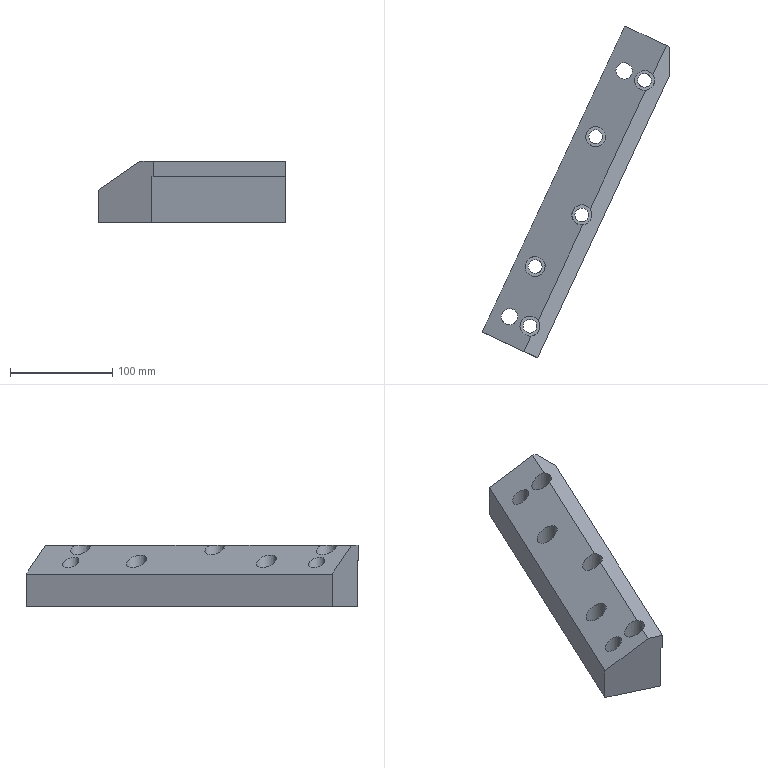Part | NX | features solid 2 | 1 solid | 27 faces | box 183.656 x 324.439 x 60 mm | volume 868161 mm3 | plane 15 | cylinder 12 | commonest cylinder face diameters 13.5 x5 19.5 x5 16 x2
STEP:
#1=CARTESIAN_POINT('',(-201.72,227.591,-65.));
#2=VERTEX_POINT('',#1);
#3=CARTESIAN_POINT('',(-201.72,234.341,-65.));
#4=DIRECTION('',(0.,0.,1.));
#5=DIRECTION('',(0.,-1.,0.));
#6=AXIS2_PLACEMENT_3D('',#3,#4,#5);
#7=CIRCLE('',#6,6.75);
#8=EDGE_CURVE('',#2,#2,#7,.T.);
#9=ORIENTED_EDGE('',*,*,#8,.T.);
#10=EDGE_LOOP('',(#9));
#11=FACE_BOUND('',#10,.T.);
#12=CARTESIAN_POINT('',(-156.124,278.049,-65.));
#13=VERTEX_POINT('',#12);
#14=CARTESIAN_POINT('',(-156.124,284.799,-65.));
#15=DIRECTION('',(0.,0.,1.));
#16=DIRECTION('',(0.,-1.,0.));
#17=AXIS2_PLACEMENT_3D('',#14,#15,#16);
#18=CIRCLE('',#17,6.75);
#19=EDGE_CURVE('',#13,#13,#18,.F.);
#20=ORIENTED_EDGE('',*,*,#19,.F.);
#21=EDGE_LOOP('',(#20));
#22=FACE_BOUND('',#21,.T.);
#23=CARTESIAN_POINT('',(-142.553,354.474,-65.));
#24=VERTEX_POINT('',#23);
#25=CARTESIAN_POINT('',(-142.553,361.224,-65.));
#26=DIRECTION('',(0.,0.,1.));
#27=DIRECTION('',(0.,-1.,0.));
#28=AXIS2_PLACEMENT_3D('',#25,#26,#27);
#29=CIRCLE('',#28,6.75);
#30=EDGE_CURVE('',#24,#24,#29,.F.);
#31=ORIENTED_EDGE('',*,*,#30,.F.);
#32=EDGE_LOOP('',(#31));
#33=FACE_BOUND('',#32,.T.);
#34=CARTESIAN_POINT('',(-94.844,409.463,-65.));
#35=VERTEX_POINT('',#34);
#36=CARTESIAN_POINT('',(-94.844,416.213,-65.));
#37=DIRECTION('',(0.,0.,1.));
#38=DIRECTION('',(0.,-1.,0.));
#39=AXIS2_PLACEMENT_3D('',#36,#37,#38);
#40=CIRCLE('',#39,6.75);
#41=EDGE_CURVE('',#35,#35,#40,.F.);
#42=ORIENTED_EDGE('',*,*,#41,.F.);
#43=EDGE_LOOP('',(#42));
#44=FACE_BOUND('',#43,.T.);
#45=CARTESIAN_POINT('',(-114.783,417.511,-65.));
#46=VERTEX_POINT('',#45);
#47=CARTESIAN_POINT('',(-114.783,425.511,-65.));
#48=DIRECTION('',(0.,0.,1.));
#49=DIRECTION('',(0.,-1.,0.));
#50=AXIS2_PLACEMENT_3D('',#47,#48,#49);
#51=CIRCLE('',#50,8.);
#52=EDGE_CURVE('',#46,#46,#51,.F.);
#53=ORIENTED_EDGE('',*,*,#52,.F.);
#54=EDGE_LOOP('',(#53));
#55=FACE_BOUND('',#54,.T.);
#56=CARTESIAN_POINT('',(-206.838,169.292,-65.));
#57=VERTEX_POINT('',#56);
#58=CARTESIAN_POINT('',(-206.838,176.042,-65.));
#59=DIRECTION('',(0.,0.,1.));
#60=DIRECTION('',(0.,-1.,0.));
#61=AXIS2_PLACEMENT_3D('',#58,#59,#60);
#62=CIRCLE('',#61,6.75);
#63=EDGE_CURVE('',#57,#57,#62,.T.);
#64=ORIENTED_EDGE('',*,*,#63,.T.);
#65=EDGE_LOOP('',(#64));
#66=FACE_BOUND('',#65,.T.);
#67=CARTESIAN_POINT('',(-226.777,177.339,-65.));
#68=VERTEX_POINT('',#67);
#69=CARTESIAN_POINT('',(-226.777,185.339,-65.));
#70=DIRECTION('',(0.,0.,1.));
#71=DIRECTION('',(0.,-1.,0.));
#72=AXIS2_PLACEMENT_3D('',#69,#70,#71);
#73=CIRCLE('',#72,8.);
#74=EDGE_CURVE('',#68,#68,#73,.T.);
#75=ORIENTED_EDGE('',*,*,#74,.T.);
#76=EDGE_LOOP('',(#75));
#77=FACE_BOUND('',#76,.T.);
#78=CARTESIAN_POINT('',(-70.,426.9,-65.));
#79=VERTEX_POINT('',#78);
#80=CARTESIAN_POINT('',(-70.,448.764,-65.));
#81=VERTEX_POINT('',#80);
#82=CARTESIAN_POINT('',(-70.,-31.798,-65.));
#83=DIRECTION('',(0.,1.,0.));
#84=VECTOR('',#83,1000.);
#85=LINE('',#82,#84);
#86=EDGE_CURVE('',#79,#81,#85,.T.);
#87=ORIENTED_EDGE('',*,*,#86,.F.);
#88=CARTESIAN_POINT('',(-201.09,145.777,-65.));
#89=VERTEX_POINT('',#88);
#90=CARTESIAN_POINT('',(-283.5,-30.953,-65.));
#91=DIRECTION('',(0.4226,0.9063,0.));
#92=VECTOR('',#91,1000.);
#93=LINE('',#90,#92);
#94=EDGE_CURVE('',#89,#79,#93,.T.);
#95=ORIENTED_EDGE('',*,*,#94,.F.);
#96=CARTESIAN_POINT('',(-253.656,170.289,-65.));
#97=VERTEX_POINT('',#96);
#98=CARTESIAN_POINT('',(-253.656,170.289,-65.));
#99=DIRECTION('',(0.9063,-0.4226,0.));
#100=VECTOR('',#99,1000.);
#101=LINE('',#98,#100);
#102=EDGE_CURVE('',#97,#89,#101,.T.);
#103=ORIENTED_EDGE('',*,*,#102,.F.);
#104=CARTESIAN_POINT('',(-114.192,469.37,-65.));
#105=VERTEX_POINT('',#104);
#106=CARTESIAN_POINT('',(-336.066,-6.441,-65.));
#107=DIRECTION('',(0.4226,0.9063,0.));
#108=VECTOR('',#107,1000.);
#109=LINE('',#106,#108);
#110=EDGE_CURVE('',#97,#105,#109,.T.);
#111=ORIENTED_EDGE('',*,*,#110,.T.);
#112=CARTESIAN_POINT('',(-59.813,444.013,-65.));
#113=DIRECTION('',(0.9063,-0.4226,0.));
#114=VECTOR('',#113,1000.);
#115=LINE('',#112,#114);
#116=EDGE_CURVE('',#81,#105,#115,.F.);
#117=ORIENTED_EDGE('',*,*,#116,.F.);
#118=EDGE_LOOP('',(#87,#95,#103,#111,#117));
#119=FACE_BOUND('',#118,.T.);
#120=CARTESIAN_POINT('',(-281.688,-31.798,-65.));
#121=DIRECTION('',(0.,0.,1.));
#122=DIRECTION('',(0.4226,0.9063,0.));
#123=AXIS2_PLACEMENT_3D('',#120,#121,#122);
#124=PLANE('',#123);
#125=ADVANCED_FACE('',(#11,#22,#33,#44,#55,#66,#77,#119),#124,.F.);
#126=CARTESIAN_POINT('',(-70.,448.764,-5.));
#127=VERTEX_POINT('',#126);
#128=CARTESIAN_POINT('',(-70.,422.168,-5.));
#129=VERTEX_POINT('',#128);
#130=CARTESIAN_POINT('',(-70.,-31.798,-5.));
#131=DIRECTION('',(0.,1.,0.));
#132=VECTOR('',#131,1000.);
#133=LINE('',#130,#132);
#134=EDGE_CURVE('',#127,#129,#133,.F.);
#135=ORIENTED_EDGE('',*,*,#134,.F.);
#136=CARTESIAN_POINT('',(-73.408,450.353,-5.));
#137=VERTEX_POINT('',#136);
#138=CARTESIAN_POINT('',(-59.813,444.013,-5.));
#139=DIRECTION('',(-0.9063,0.4226,0.));
#140=VECTOR('',#139,1000.);
#141=LINE('',#138,#140);
#142=EDGE_CURVE('',#127,#137,#141,.T.);
#143=ORIENTED_EDGE('',*,*,#142,.T.);
#144=CARTESIAN_POINT('',(-86.775,421.686,-5.));
#145=VERTEX_POINT('',#144);
#146=CARTESIAN_POINT('',(-295.282,-25.459,-5.));
#147=DIRECTION('',(-0.4226,-0.9063,0.));
#148=VECTOR('',#147,1000.);
#149=LINE('',#146,#148);
#150=EDGE_CURVE('',#145,#137,#149,.F.);
#151=ORIENTED_EDGE('',*,*,#150,.F.);
#152=CARTESIAN_POINT('',(-93.85,406.514,-5.));
#153=VERTEX_POINT('',#152);
#154=CARTESIAN_POINT('',(-94.844,416.213,-5.));
#155=DIRECTION('',(0.,0.,-1.));
#156=DIRECTION('',(0.4226,0.9063,0.));
#157=AXIS2_PLACEMENT_3D('',#154,#155,#156);
#158=CIRCLE('',#157,9.75);
#159=EDGE_CURVE('',#153,#145,#158,.F.);
#160=ORIENTED_EDGE('',*,*,#159,.F.);
#161=CARTESIAN_POINT('',(-148.055,290.272,-5.));
#162=VERTEX_POINT('',#161);
#163=CARTESIAN_POINT('',(-295.282,-25.459,-5.));
#164=DIRECTION('',(-0.4226,-0.9063,0.));
#165=VECTOR('',#164,1000.);
#166=LINE('',#163,#165);
#167=EDGE_CURVE('',#162,#153,#166,.F.);
#168=ORIENTED_EDGE('',*,*,#167,.F.);
#169=CARTESIAN_POINT('',(-155.13,275.1,-5.));
#170=VERTEX_POINT('',#169);
#171=CARTESIAN_POINT('',(-156.124,284.799,-5.));
#172=DIRECTION('',(0.,0.,-1.));
#173=DIRECTION('',(0.4226,0.9063,0.));
#174=AXIS2_PLACEMENT_3D('',#171,#172,#173);
#175=CIRCLE('',#174,9.75);
#176=EDGE_CURVE('',#170,#162,#175,.F.);
#177=ORIENTED_EDGE('',*,*,#176,.F.);
#178=CARTESIAN_POINT('',(-198.769,181.515,-5.));
#179=VERTEX_POINT('',#178);
#180=CARTESIAN_POINT('',(-295.282,-25.459,-5.));
#181=DIRECTION('',(-0.4226,-0.9063,0.));
#182=VECTOR('',#181,1000.);
#183=LINE('',#180,#182);
#184=EDGE_CURVE('',#179,#170,#183,.F.);
#185=ORIENTED_EDGE('',*,*,#184,.F.);
#186=CARTESIAN_POINT('',(-205.844,166.343,-5.));
#187=VERTEX_POINT('',#186);
#188=CARTESIAN_POINT('',(-206.838,176.042,-5.));
#189=DIRECTION('',(0.,0.,-1.));
#190=DIRECTION('',(0.4226,0.9063,0.));
#191=AXIS2_PLACEMENT_3D('',#188,#189,#190);
#192=CIRCLE('',#191,9.75);
#193=EDGE_CURVE('',#187,#179,#192,.F.);
#194=ORIENTED_EDGE('',*,*,#193,.F.);
#195=CARTESIAN_POINT('',(-212.872,151.271,-5.));
#196=VERTEX_POINT('',#195);
#197=CARTESIAN_POINT('',(-295.282,-25.459,-5.));
#198=DIRECTION('',(-0.4226,-0.9063,0.));
#199=VECTOR('',#198,1000.);
#200=LINE('',#197,#199);
#201=EDGE_CURVE('',#196,#187,#200,.F.);
#202=ORIENTED_EDGE('',*,*,#201,.F.);
#203=CARTESIAN_POINT('',(-199.277,144.932,-5.));
#204=VERTEX_POINT('',#203);
#205=CARTESIAN_POINT('',(-199.277,144.932,-5.));
#206=DIRECTION('',(0.9063,-0.4226,0.));
#207=VECTOR('',#206,1000.);
#208=LINE('',#205,#207);
#209=EDGE_CURVE('',#204,#196,#208,.F.);
#210=ORIENTED_EDGE('',*,*,#209,.F.);
#211=CARTESIAN_POINT('',(-281.688,-31.798,-5.));
#212=DIRECTION('',(0.4226,0.9063,0.));
#213=VECTOR('',#212,1000.);
#214=LINE('',#211,#213);
#215=EDGE_CURVE('',#204,#129,#214,.T.);
#216=ORIENTED_EDGE('',*,*,#215,.T.);
#217=EDGE_LOOP('',(#135,#143,#151,#160,#168,#177,#185,#194,#202,#210,#216));
#218=FACE_BOUND('',#217,.T.);
#219=CARTESIAN_POINT('',(-281.688,-31.798,-5.));
#220=DIRECTION('',(0.,0.,1.));
#221=DIRECTION('',(0.4226,0.9063,0.));
#222=AXIS2_PLACEMENT_3D('',#219,#220,#221);
#223=PLANE('',#222);
#224=ADVANCED_FACE('',(#218),#223,.T.);
#225=CARTESIAN_POINT('',(-199.277,144.932,-20.));
#226=VERTEX_POINT('',#225);
#227=CARTESIAN_POINT('',(-70.,422.168,-20.));
#228=VERTEX_POINT('',#227);
#229=CARTESIAN_POINT('',(-281.688,-31.798,-20.));
#230=DIRECTION('',(0.4226,0.9063,0.));
#231=VECTOR('',#230,1000.);
#232=LINE('',#229,#231);
#233=EDGE_CURVE('',#226,#228,#232,.T.);
#234=ORIENTED_EDGE('',*,*,#233,.T.);
#235=CARTESIAN_POINT('',(-70.,422.168,-5.));
#236=DIRECTION('',(0.,0.,1.));
#237=VECTOR('',#236,1000.);
#238=LINE('',#235,#237);
#239=EDGE_CURVE('',#228,#129,#238,.T.);
#240=ORIENTED_EDGE('',*,*,#239,.T.);
#241=ORIENTED_EDGE('',*,*,#215,.F.);
#242=CARTESIAN_POINT('',(-199.277,144.932,-5.));
#243=DIRECTION('',(0.,0.,-1.));
#244=VECTOR('',#243,1000.);
#245=LINE('',#242,#244);
#246=EDGE_CURVE('',#204,#226,#245,.T.);
#247=ORIENTED_EDGE('',*,*,#246,.T.);
#248=EDGE_LOOP('',(#234,#240,#241,#247));
#249=FACE_BOUND('',#248,.T.);
#250=CARTESIAN_POINT('',(-281.688,-31.798,-5.));
#251=DIRECTION('',(0.9063,-0.4226,0.));
#252=DIRECTION('',(-0.4226,-0.9063,0.));
#253=AXIS2_PLACEMENT_3D('',#250,#251,#252);
#254=PLANE('',#253);
#255=ADVANCED_FACE('',(#249),#254,.T.);
#256=CARTESIAN_POINT('',(-70.,426.9,-20.));
#257=VERTEX_POINT('',#256);
#258=CARTESIAN_POINT('',(-70.,-31.798,-20.));
#259=DIRECTION('',(0.,-1.,0.));
#260=VECTOR('',#259,1000.);
#261=LINE('',#258,#260);
#262=EDGE_CURVE('',#228,#257,#261,.F.);
#263=ORIENTED_EDGE('',*,*,#262,.F.);
#264=ORIENTED_EDGE('',*,*,#233,.F.);
#265=CARTESIAN_POINT('',(-201.09,145.777,-20.));
#266=VERTEX_POINT('',#265);
#267=CARTESIAN_POINT('',(-199.277,144.932,-20.));
#268=DIRECTION('',(-0.9063,0.4226,0.));
#269=VECTOR('',#268,1000.);
#270=LINE('',#267,#269);
#271=EDGE_CURVE('',#266,#226,#270,.F.);
#272=ORIENTED_EDGE('',*,*,#271,.F.);
#273=CARTESIAN_POINT('',(-283.5,-30.953,-20.));
#274=DIRECTION('',(0.4226,0.9063,0.));
#275=VECTOR('',#274,1000.);
#276=LINE('',#273,#275);
#277=EDGE_CURVE('',#266,#257,#276,.T.);
#278=ORIENTED_EDGE('',*,*,#277,.T.);
#279=EDGE_LOOP('',(#263,#264,#272,#278));
#280=FACE_BOUND('',#279,.T.);
#281=CARTESIAN_POINT('',(-281.688,-31.798,-20.));
#282=DIRECTION('',(0.,0.,-1.));
#283=DIRECTION('',(0.4226,0.9063,0.));
#284=AXIS2_PLACEMENT_3D('',#281,#282,#283);
#285=PLANE('',#284);
#286=ADVANCED_FACE('',(#280),#285,.T.);
#287=CARTESIAN_POINT('',(-70.,426.9,-55.));
#288=DIRECTION('',(0.,0.,-1.));
#289=VECTOR('',#288,1000.);
#290=LINE('',#287,#289);
#291=EDGE_CURVE('',#257,#79,#290,.T.);
#292=ORIENTED_EDGE('',*,*,#291,.F.);
#293=ORIENTED_EDGE('',*,*,#277,.F.);
#294=CARTESIAN_POINT('',(-201.09,145.777,-55.));
#295=DIRECTION('',(0.,0.,1.));
#296=VECTOR('',#295,1000.);
#297=LINE('',#294,#296);
#298=EDGE_CURVE('',#89,#266,#297,.T.);
#299=ORIENTED_EDGE('',*,*,#298,.F.);
#300=ORIENTED_EDGE('',*,*,#94,.T.);
#301=EDGE_LOOP('',(#292,#293,#299,#300));
#302=FACE_BOUND('',#301,.T.);
#303=CARTESIAN_POINT('',(-283.5,-30.953,-55.));
#304=DIRECTION('',(-0.9063,0.4226,0.));
#305=DIRECTION('',(0.4226,0.9063,0.));
#306=AXIS2_PLACEMENT_3D('',#303,#304,#305);
#307=PLANE('',#306);
#308=ADVANCED_FACE('',(#302),#307,.F.);
#309=CARTESIAN_POINT('',(-70.,448.764,-5.));
#310=DIRECTION('',(0.,0.,-1.));
#311=VECTOR('',#310,1000.);
#312=LINE('',#309,#311);
#313=EDGE_CURVE('',#81,#127,#312,.F.);
#314=ORIENTED_EDGE('',*,*,#313,.F.);
#315=ORIENTED_EDGE('',*,*,#116,.T.);
#316=CARTESIAN_POINT('',(-114.192,469.37,-33.125));
#317=VERTEX_POINT('',#316);
#318=CARTESIAN_POINT('',(-114.192,469.37,-5.));
#319=DIRECTION('',(0.,0.,-1.));
#320=VECTOR('',#319,1000.);
#321=LINE('',#318,#320);
#322=EDGE_CURVE('',#105,#317,#321,.F.);
#323=ORIENTED_EDGE('',*,*,#322,.T.);
#324=CARTESIAN_POINT('',(-63.632,445.794,1.742));
#325=DIRECTION('',(0.7685,-0.3584,0.53));
#326=VECTOR('',#325,1000.);
#327=LINE('',#324,#326);
#328=EDGE_CURVE('',#137,#317,#327,.F.);
#329=ORIENTED_EDGE('',*,*,#328,.F.);
#330=ORIENTED_EDGE('',*,*,#142,.F.);
#331=EDGE_LOOP('',(#314,#315,#323,#329,#330));
#332=FACE_BOUND('',#331,.T.);
#333=CARTESIAN_POINT('',(-59.813,444.013,-5.));
#334=DIRECTION('',(0.4226,0.9063,0.));
#335=DIRECTION('',(0.,0.,-1.));
#336=AXIS2_PLACEMENT_3D('',#333,#334,#335);
#337=PLANE('',#336);
#338=ADVANCED_FACE('',(#332),#337,.T.);
#339=CARTESIAN_POINT('',(-234.027,188.72,-26.875));
#340=VERTEX_POINT('',#339);
#341=CARTESIAN_POINT('',(-226.777,185.339,-21.875));
#342=DIRECTION('',(-0.4803,0.224,0.848));
#343=DIRECTION('',(-0.7685,0.3584,-0.53));
#344=AXIS2_PLACEMENT_3D('',#341,#342,#343);
#345=ELLIPSE('',#344,9.434,8.);
#346=EDGE_CURVE('',#340,#340,#345,.F.);
#347=ORIENTED_EDGE('',*,*,#346,.T.);
#348=EDGE_LOOP('',(#347));
#349=FACE_BOUND('',#348,.T.);
#350=CARTESIAN_POINT('',(-210.557,238.462,-26.719));
#351=VERTEX_POINT('',#350);
#352=CARTESIAN_POINT('',(-201.72,234.341,-20.625));
#353=DIRECTION('',(-0.4803,0.224,0.848));
#354=DIRECTION('',(-0.7685,0.3584,-0.53));
#355=AXIS2_PLACEMENT_3D('',#352,#353,#354);
#356=ELLIPSE('',#355,11.498,9.75);
#357=EDGE_CURVE('',#351,#351,#356,.F.);
#358=ORIENTED_EDGE('',*,*,#357,.T.);
#359=EDGE_LOOP('',(#358));
#360=FACE_BOUND('',#359,.T.);
#361=CARTESIAN_POINT('',(-206.838,176.042,-8.125));
#362=DIRECTION('',(-0.4803,0.224,0.848));
#363=DIRECTION('',(-0.7685,0.3584,-0.53));
#364=AXIS2_PLACEMENT_3D('',#361,#362,#363);
#365=ELLIPSE('',#364,11.498,9.75);
#366=EDGE_CURVE('',#187,#179,#365,.F.);
#367=ORIENTED_EDGE('',*,*,#366,.T.);
#368=ORIENTED_EDGE('',*,*,#184,.T.);
#369=CARTESIAN_POINT('',(-156.124,284.799,-8.125));
#370=DIRECTION('',(-0.4803,0.224,0.848));
#371=DIRECTION('',(-0.7685,0.3584,-0.53));
#372=AXIS2_PLACEMENT_3D('',#369,#370,#371);
#373=ELLIPSE('',#372,11.498,9.75);
#374=EDGE_CURVE('',#170,#162,#373,.F.);
#375=ORIENTED_EDGE('',*,*,#374,.T.);
#376=ORIENTED_EDGE('',*,*,#167,.T.);
#377=CARTESIAN_POINT('',(-94.844,416.213,-8.125));
#378=DIRECTION('',(-0.4803,0.224,0.848));
#379=DIRECTION('',(-0.7685,0.3584,-0.53));
#380=AXIS2_PLACEMENT_3D('',#377,#378,#379);
#381=ELLIPSE('',#380,11.498,9.75);
#382=EDGE_CURVE('',#153,#145,#381,.F.);
#383=ORIENTED_EDGE('',*,*,#382,.T.);
#384=ORIENTED_EDGE('',*,*,#150,.T.);
#385=ORIENTED_EDGE('',*,*,#328,.T.);
#386=CARTESIAN_POINT('',(-253.656,170.289,-33.125));
#387=VERTEX_POINT('',#386);
#388=CARTESIAN_POINT('',(-336.066,-6.441,-33.125));
#389=DIRECTION('',(-0.4226,-0.9063,0.));
#390=VECTOR('',#389,1000.);
#391=LINE('',#388,#390);
#392=EDGE_CURVE('',#317,#387,#391,.T.);
#393=ORIENTED_EDGE('',*,*,#392,.T.);
#394=CARTESIAN_POINT('',(-212.872,151.271,-5.));
#395=DIRECTION('',(0.7685,-0.3584,0.53));
#396=VECTOR('',#395,1000.);
#397=LINE('',#394,#396);
#398=EDGE_CURVE('',#387,#196,#397,.T.);
#399=ORIENTED_EDGE('',*,*,#398,.T.);
#400=ORIENTED_EDGE('',*,*,#201,.T.);
#401=EDGE_LOOP('',(#367,#368,#375,#376,#383,#384,#385,#393,#399,#400));
#402=FACE_BOUND('',#401,.T.);
#403=CARTESIAN_POINT('',(-151.39,365.345,-26.719));
#404=VERTEX_POINT('',#403);
#405=CARTESIAN_POINT('',(-142.553,361.224,-20.625));
#406=DIRECTION('',(-0.4803,0.224,0.848));
#407=DIRECTION('',(-0.7685,0.3584,-0.53));
#408=AXIS2_PLACEMENT_3D('',#405,#406,#407);
#409=ELLIPSE('',#408,11.498,9.75);
#410=EDGE_CURVE('',#404,#404,#409,.F.);
#411=ORIENTED_EDGE('',*,*,#410,.T.);
#412=EDGE_LOOP('',(#411));
#413=FACE_BOUND('',#412,.T.);
#414=CARTESIAN_POINT('',(-122.033,428.892,-26.875));
#415=VERTEX_POINT('',#414);
#416=CARTESIAN_POINT('',(-114.783,425.511,-21.875));
#417=DIRECTION('',(-0.4803,0.224,0.848));
#418=DIRECTION('',(-0.7685,0.3584,-0.53));
#419=AXIS2_PLACEMENT_3D('',#416,#417,#418);
#420=ELLIPSE('',#419,9.434,8.);
#421=EDGE_CURVE('',#415,#415,#420,.F.);
#422=ORIENTED_EDGE('',*,*,#421,.T.);
#423=EDGE_LOOP('',(#422));
#424=FACE_BOUND('',#423,.T.);
#425=CARTESIAN_POINT('',(-295.282,-25.459,-5.));
#426=DIRECTION('',(-0.4803,0.224,0.848));
#427=DIRECTION('',(0.7685,-0.3584,0.53));
#428=AXIS2_PLACEMENT_3D('',#425,#426,#427);
#429=PLANE('',#428);
#430=ADVANCED_FACE('',(#349,#360,#402,#413,#424),#429,.T.);
#431=ORIENTED_EDGE('',*,*,#322,.F.);
#432=ORIENTED_EDGE('',*,*,#110,.F.);
#433=CARTESIAN_POINT('',(-253.656,170.289,-30.));
#434=DIRECTION('',(0.,0.,-1.));
#435=VECTOR('',#434,1000.);
#436=LINE('',#433,#435);
#437=EDGE_CURVE('',#387,#97,#436,.T.);
#438=ORIENTED_EDGE('',*,*,#437,.F.);
#439=ORIENTED_EDGE('',*,*,#392,.F.);
#440=EDGE_LOOP('',(#431,#432,#438,#439));
#441=FACE_BOUND('',#440,.T.);
#442=CARTESIAN_POINT('',(-336.066,-6.441,-5.));
#443=DIRECTION('',(0.9063,-0.4226,0.));
#444=DIRECTION('',(-0.4226,-0.9063,0.));
#445=AXIS2_PLACEMENT_3D('',#442,#443,#444);
#446=PLANE('',#445);
#447=ADVANCED_FACE('',(#441),#446,.F.);
#448=CARTESIAN_POINT('',(-162.874,284.799,-40.));
#449=VERTEX_POINT('',#448);
#450=CARTESIAN_POINT('',(-156.124,284.799,-40.));
#451=DIRECTION('',(0.,0.,-1.));
#452=DIRECTION('',(-1.,0.,0.));
#453=AXIS2_PLACEMENT_3D('',#450,#451,#452);
#454=CIRCLE('',#453,6.75);
#455=EDGE_CURVE('',#449,#449,#454,.T.);
#456=ORIENTED_EDGE('',*,*,#455,.F.);
#457=EDGE_LOOP('',(#456));
#458=FACE_BOUND('',#457,.T.);
#459=ORIENTED_EDGE('',*,*,#19,.T.);
#460=EDGE_LOOP('',(#459));
#461=FACE_BOUND('',#460,.T.);
#462=CARTESIAN_POINT('',(-156.124,284.799,70.));
#463=DIRECTION('',(0.,0.,-1.));
#464=DIRECTION('',(-0.9063,0.4226,0.));
#465=AXIS2_PLACEMENT_3D('',#462,#463,#464);
#466=CYLINDRICAL_SURFACE('',#465,6.75);
#467=ADVANCED_FACE('',(#458,#461),#466,.F.);
#468=CARTESIAN_POINT('',(-149.303,361.224,-40.));
#469=VERTEX_POINT('',#468);
#470=CARTESIAN_POINT('',(-142.553,361.224,-40.));
#471=DIRECTION('',(0.,0.,-1.));
#472=DIRECTION('',(-1.,0.,0.));
#473=AXIS2_PLACEMENT_3D('',#470,#471,#472);
#474=CIRCLE('',#473,6.75);
#475=EDGE_CURVE('',#469,#469,#474,.T.);
#476=ORIENTED_EDGE('',*,*,#475,.F.);
#477=EDGE_LOOP('',(#476));
#478=FACE_BOUND('',#477,.T.);
#479=ORIENTED_EDGE('',*,*,#30,.T.);
#480=EDGE_LOOP('',(#479));
#481=FACE_BOUND('',#480,.T.);
#482=CARTESIAN_POINT('',(-142.553,361.224,70.));
#483=DIRECTION('',(0.,0.,-1.));
#484=DIRECTION('',(-0.9063,0.4226,0.));
#485=AXIS2_PLACEMENT_3D('',#482,#483,#484);
#486=CYLINDRICAL_SURFACE('',#485,6.75);
#487=ADVANCED_FACE('',(#478,#481),#486,.F.);
#488=CARTESIAN_POINT('',(-101.594,416.213,-40.));
#489=VERTEX_POINT('',#488);
#490=CARTESIAN_POINT('',(-94.844,416.213,-40.));
#491=DIRECTION('',(0.,0.,-1.));
#492=DIRECTION('',(-1.,0.,0.));
#493=AXIS2_PLACEMENT_3D('',#490,#491,#492);
#494=CIRCLE('',#493,6.75);
#495=EDGE_CURVE('',#489,#489,#494,.T.);
#496=ORIENTED_EDGE('',*,*,#495,.F.);
#497=EDGE_LOOP('',(#496));
#498=FACE_BOUND('',#497,.T.);
#499=ORIENTED_EDGE('',*,*,#41,.T.);
#500=EDGE_LOOP('',(#499));
#501=FACE_BOUND('',#500,.T.);
#502=CARTESIAN_POINT('',(-94.844,416.213,70.));
#503=DIRECTION('',(0.,0.,-1.));
#504=DIRECTION('',(-0.9063,0.4226,0.));
#505=AXIS2_PLACEMENT_3D('',#502,#503,#504);
#506=CYLINDRICAL_SURFACE('',#505,6.75);
#507=ADVANCED_FACE('',(#498,#501),#506,.F.);
#508=ORIENTED_EDGE('',*,*,#421,.F.);
#509=EDGE_LOOP('',(#508));
#510=FACE_BOUND('',#509,.T.);
#511=ORIENTED_EDGE('',*,*,#52,.T.);
#512=EDGE_LOOP('',(#511));
#513=FACE_BOUND('',#512,.T.);
#514=CARTESIAN_POINT('',(-114.783,425.511,45.));
#515=DIRECTION('',(0.,0.,-1.));
#516=DIRECTION('',(-0.9063,0.4226,0.));
#517=AXIS2_PLACEMENT_3D('',#514,#515,#516);
#518=CYLINDRICAL_SURFACE('',#517,8.);
#519=ADVANCED_FACE('',(#510,#513),#518,.F.);
#520=CARTESIAN_POINT('',(-104.594,416.213,-40.));
#521=VERTEX_POINT('',#520);
#522=CARTESIAN_POINT('',(-94.844,416.213,-40.));
#523=DIRECTION('',(0.,0.,-1.));
#524=DIRECTION('',(-1.,0.,0.));
#525=AXIS2_PLACEMENT_3D('',#522,#523,#524);
#526=CIRCLE('',#525,9.75);
#527=EDGE_CURVE('',#521,#521,#526,.F.);
#528=ORIENTED_EDGE('',*,*,#527,.F.);
#529=EDGE_LOOP('',(#528));
#530=FACE_BOUND('',#529,.T.);
#531=ORIENTED_EDGE('',*,*,#382,.F.);
#532=ORIENTED_EDGE('',*,*,#159,.T.);
#533=EDGE_LOOP('',(#531,#532));
#534=FACE_BOUND('',#533,.T.);
#535=CARTESIAN_POINT('',(-94.844,416.213,70.));
#536=DIRECTION('',(0.,0.,-1.));
#537=DIRECTION('',(-0.9063,0.4226,0.));
#538=AXIS2_PLACEMENT_3D('',#535,#536,#537);
#539=CYLINDRICAL_SURFACE('',#538,9.75);
#540=ADVANCED_FACE('',(#530,#534),#539,.F.);
#541=ORIENTED_EDGE('',*,*,#527,.T.);
#542=EDGE_LOOP('',(#541));
#543=FACE_BOUND('',#542,.T.);
#544=ORIENTED_EDGE('',*,*,#495,.T.);
#545=EDGE_LOOP('',(#544));
#546=FACE_BOUND('',#545,.T.);
#547=CARTESIAN_POINT('',(-94.844,416.213,-40.));
#548=DIRECTION('',(0.,0.,-1.));
#549=DIRECTION('',(-0.9063,0.4226,0.));
#550=AXIS2_PLACEMENT_3D('',#547,#548,#549);
#551=PLANE('',#550);
#552=ADVANCED_FACE('',(#543,#546),#551,.F.);
#553=CARTESIAN_POINT('',(-152.303,361.224,-40.));
#554=VERTEX_POINT('',#553);
#555=CARTESIAN_POINT('',(-142.553,361.224,-40.));
#556=DIRECTION('',(0.,0.,-1.));
#557=DIRECTION('',(-1.,0.,0.));
#558=AXIS2_PLACEMENT_3D('',#555,#556,#557);
#559=CIRCLE('',#558,9.75);
#560=EDGE_CURVE('',#554,#554,#559,.F.);
#561=ORIENTED_EDGE('',*,*,#560,.T.);
#562=EDGE_LOOP('',(#561));
#563=FACE_BOUND('',#562,.T.);
#564=ORIENTED_EDGE('',*,*,#475,.T.);
#565=EDGE_LOOP('',(#564));
#566=FACE_BOUND('',#565,.T.);
#567=CARTESIAN_POINT('',(-142.553,361.224,-40.));
#568=DIRECTION('',(0.,0.,-1.));
#569=DIRECTION('',(-0.9063,0.4226,0.));
#570=AXIS2_PLACEMENT_3D('',#567,#568,#569);
#571=PLANE('',#570);
#572=ADVANCED_FACE('',(#563,#566),#571,.F.);
#573=ORIENTED_EDGE('',*,*,#410,.F.);
#574=EDGE_LOOP('',(#573));
#575=FACE_BOUND('',#574,.T.);
#576=ORIENTED_EDGE('',*,*,#560,.F.);
#577=EDGE_LOOP('',(#576));
#578=FACE_BOUND('',#577,.T.);
#579=CARTESIAN_POINT('',(-142.553,361.224,70.));
#580=DIRECTION('',(0.,0.,-1.));
#581=DIRECTION('',(-0.9063,0.4226,0.));
#582=AXIS2_PLACEMENT_3D('',#579,#580,#581);
#583=CYLINDRICAL_SURFACE('',#582,9.75);
#584=ADVANCED_FACE('',(#575,#578),#583,.F.);
#585=CARTESIAN_POINT('',(-165.874,284.799,-40.));
#586=VERTEX_POINT('',#585);
#587=CARTESIAN_POINT('',(-156.124,284.799,-40.));
#588=DIRECTION('',(0.,0.,-1.));
#589=DIRECTION('',(-1.,0.,0.));
#590=AXIS2_PLACEMENT_3D('',#587,#588,#589);
#591=CIRCLE('',#590,9.75);
#592=EDGE_CURVE('',#586,#586,#591,.F.);
#593=ORIENTED_EDGE('',*,*,#592,.F.);
#594=EDGE_LOOP('',(#593));
#595=FACE_BOUND('',#594,.T.);
#596=ORIENTED_EDGE('',*,*,#374,.F.);
#597=ORIENTED_EDGE('',*,*,#176,.T.);
#598=EDGE_LOOP('',(#596,#597));
#599=FACE_BOUND('',#598,.T.);
#600=CARTESIAN_POINT('',(-156.124,284.799,70.));
#601=DIRECTION('',(0.,0.,-1.));
#602=DIRECTION('',(-0.9063,0.4226,0.));
#603=AXIS2_PLACEMENT_3D('',#600,#601,#602);
#604=CYLINDRICAL_SURFACE('',#603,9.75);
#605=ADVANCED_FACE('',(#595,#599),#604,.F.);
#606=ORIENTED_EDGE('',*,*,#592,.T.);
#607=EDGE_LOOP('',(#606));
#608=FACE_BOUND('',#607,.T.);
#609=ORIENTED_EDGE('',*,*,#455,.T.);
#610=EDGE_LOOP('',(#609));
#611=FACE_BOUND('',#610,.T.);
#612=CARTESIAN_POINT('',(-156.124,284.799,-40.));
#613=DIRECTION('',(0.,0.,-1.));
#614=DIRECTION('',(-0.9063,0.4226,0.));
#615=AXIS2_PLACEMENT_3D('',#612,#613,#614);
#616=PLANE('',#615);
#617=ADVANCED_FACE('',(#608,#611),#616,.F.);
#618=ORIENTED_EDGE('',*,*,#437,.T.);
#619=ORIENTED_EDGE('',*,*,#102,.T.);
#620=ORIENTED_EDGE('',*,*,#298,.T.);
#621=ORIENTED_EDGE('',*,*,#271,.T.);
#622=ORIENTED_EDGE('',*,*,#246,.F.);
#623=ORIENTED_EDGE('',*,*,#209,.T.);
#624=ORIENTED_EDGE('',*,*,#398,.F.);
#625=EDGE_LOOP('',(#618,#619,#620,#621,#622,#623,#624));
#626=FACE_BOUND('',#625,.T.);
#627=CARTESIAN_POINT('',(-253.656,170.289,-30.));
#628=DIRECTION('',(0.4226,0.9063,0.));
#629=DIRECTION('',(0.,0.,-1.));
#630=AXIS2_PLACEMENT_3D('',#627,#628,#629);
#631=PLANE('',#630);
#632=ADVANCED_FACE('',(#626),#631,.F.);
#633=CARTESIAN_POINT('',(-213.588,176.042,-40.));
#634=VERTEX_POINT('',#633);
#635=CARTESIAN_POINT('',(-206.838,176.042,-40.));
#636=DIRECTION('',(0.,0.,-1.));
#637=DIRECTION('',(-1.,0.,0.));
#638=AXIS2_PLACEMENT_3D('',#635,#636,#637);
#639=CIRCLE('',#638,6.75);
#640=EDGE_CURVE('',#634,#634,#639,.F.);
#641=ORIENTED_EDGE('',*,*,#640,.T.);
#642=EDGE_LOOP('',(#641));
#643=FACE_BOUND('',#642,.T.);
#644=ORIENTED_EDGE('',*,*,#63,.F.);
#645=EDGE_LOOP('',(#644));
#646=FACE_BOUND('',#645,.T.);
#647=CARTESIAN_POINT('',(-206.838,176.042,470.));
#648=DIRECTION('',(0.,0.,-1.));
#649=DIRECTION('',(-0.9063,0.4226,0.));
#650=AXIS2_PLACEMENT_3D('',#647,#648,#649);
#651=CYLINDRICAL_SURFACE('',#650,6.75);
#652=ADVANCED_FACE('',(#643,#646),#651,.F.);
#653=CARTESIAN_POINT('',(-208.47,234.341,-40.));
#654=VERTEX_POINT('',#653);
#655=CARTESIAN_POINT('',(-201.72,234.341,-40.));
#656=DIRECTION('',(0.,0.,-1.));
#657=DIRECTION('',(-1.,0.,0.));
#658=AXIS2_PLACEMENT_3D('',#655,#656,#657);
#659=CIRCLE('',#658,6.75);
#660=EDGE_CURVE('',#654,#654,#659,.F.);
#661=ORIENTED_EDGE('',*,*,#660,.T.);
#662=EDGE_LOOP('',(#661));
#663=FACE_BOUND('',#662,.T.);
#664=ORIENTED_EDGE('',*,*,#8,.F.);
#665=EDGE_LOOP('',(#664));
#666=FACE_BOUND('',#665,.T.);
#667=CARTESIAN_POINT('',(-201.72,234.341,470.));
#668=DIRECTION('',(0.,0.,-1.));
#669=DIRECTION('',(-0.9063,0.4226,0.));
#670=AXIS2_PLACEMENT_3D('',#667,#668,#669);
#671=CYLINDRICAL_SURFACE('',#670,6.75);
#672=ADVANCED_FACE('',(#663,#666),#671,.F.);
#673=ORIENTED_EDGE('',*,*,#366,.F.);
#674=ORIENTED_EDGE('',*,*,#193,.T.);
#675=EDGE_LOOP('',(#673,#674));
#676=FACE_BOUND('',#675,.T.);
#677=CARTESIAN_POINT('',(-216.588,176.042,-40.));
#678=VERTEX_POINT('',#677);
#679=CARTESIAN_POINT('',(-206.838,176.042,-40.));
#680=DIRECTION('',(0.,0.,-1.));
#681=DIRECTION('',(-1.,0.,0.));
#682=AXIS2_PLACEMENT_3D('',#679,#680,#681);
#683=CIRCLE('',#682,9.75);
#684=EDGE_CURVE('',#678,#678,#683,.F.);
#685=ORIENTED_EDGE('',*,*,#684,.F.);
#686=EDGE_LOOP('',(#685));
#687=FACE_BOUND('',#686,.T.);
#688=CARTESIAN_POINT('',(-206.838,176.042,470.));
#689=DIRECTION('',(0.,0.,-1.));
#690=DIRECTION('',(-0.9063,0.4226,0.));
#691=AXIS2_PLACEMENT_3D('',#688,#689,#690);
#692=CYLINDRICAL_SURFACE('',#691,9.75);
#693=ADVANCED_FACE('',(#676,#687),#692,.F.);
#694=ORIENTED_EDGE('',*,*,#640,.F.);
#695=EDGE_LOOP('',(#694));
#696=FACE_BOUND('',#695,.T.);
#697=ORIENTED_EDGE('',*,*,#684,.T.);
#698=EDGE_LOOP('',(#697));
#699=FACE_BOUND('',#698,.T.);
#700=CARTESIAN_POINT('',(-206.838,176.042,-40.));
#701=DIRECTION('',(0.,0.,-1.));
#702=DIRECTION('',(-0.9063,0.4226,0.));
#703=AXIS2_PLACEMENT_3D('',#700,#701,#702);
#704=PLANE('',#703);
#705=ADVANCED_FACE('',(#696,#699),#704,.F.);
#706=ORIENTED_EDGE('',*,*,#357,.F.);
#707=EDGE_LOOP('',(#706));
#708=FACE_BOUND('',#707,.T.);
#709=CARTESIAN_POINT('',(-211.47,234.341,-40.));
#710=VERTEX_POINT('',#709);
#711=CARTESIAN_POINT('',(-201.72,234.341,-40.));
#712=DIRECTION('',(0.,0.,-1.));
#713=DIRECTION('',(-1.,0.,0.));
#714=AXIS2_PLACEMENT_3D('',#711,#712,#713);
#715=CIRCLE('',#714,9.75);
#716=EDGE_CURVE('',#710,#710,#715,.F.);
#717=ORIENTED_EDGE('',*,*,#716,.F.);
#718=EDGE_LOOP('',(#717));
#719=FACE_BOUND('',#718,.T.);
#720=CARTESIAN_POINT('',(-201.72,234.341,470.));
#721=DIRECTION('',(0.,0.,-1.));
#722=DIRECTION('',(-0.9063,0.4226,0.));
#723=AXIS2_PLACEMENT_3D('',#720,#721,#722);
#724=CYLINDRICAL_SURFACE('',#723,9.75);
#725=ADVANCED_FACE('',(#708,#719),#724,.F.);
#726=ORIENTED_EDGE('',*,*,#660,.F.);
#727=EDGE_LOOP('',(#726));
#728=FACE_BOUND('',#727,.T.);
#729=ORIENTED_EDGE('',*,*,#716,.T.);
#730=EDGE_LOOP('',(#729));
#731=FACE_BOUND('',#730,.T.);
#732=CARTESIAN_POINT('',(-201.72,234.341,-40.));
#733=DIRECTION('',(0.,0.,-1.));
#734=DIRECTION('',(-0.9063,0.4226,0.));
#735=AXIS2_PLACEMENT_3D('',#732,#733,#734);
#736=PLANE('',#735);
#737=ADVANCED_FACE('',(#728,#731),#736,.F.);
#738=ORIENTED_EDGE('',*,*,#346,.F.);
#739=EDGE_LOOP('',(#738));
#740=FACE_BOUND('',#739,.T.);
#741=ORIENTED_EDGE('',*,*,#74,.F.);
#742=EDGE_LOOP('',(#741));
#743=FACE_BOUND('',#742,.T.);
#744=CARTESIAN_POINT('',(-226.777,185.339,445.));
#745=DIRECTION('',(0.,0.,-1.));
#746=DIRECTION('',(-0.9063,0.4226,0.));
#747=AXIS2_PLACEMENT_3D('',#744,#745,#746);
#748=CYLINDRICAL_SURFACE('',#747,8.);
#749=ADVANCED_FACE('',(#740,#743),#748,.F.);
#750=ORIENTED_EDGE('',*,*,#239,.F.);
#751=ORIENTED_EDGE('',*,*,#262,.T.);
#752=ORIENTED_EDGE('',*,*,#291,.T.);
#753=ORIENTED_EDGE('',*,*,#86,.T.);
#754=ORIENTED_EDGE('',*,*,#313,.T.);
#755=ORIENTED_EDGE('',*,*,#134,.T.);
#756=EDGE_LOOP('',(#750,#751,#752,#753,#754,#755));
#757=FACE_BOUND('',#756,.T.);
#758=CARTESIAN_POINT('',(-70.,0.,0.));
#759=DIRECTION('',(1.,0.,0.));
#760=DIRECTION('',(0.,0.,-1.));
#761=AXIS2_PLACEMENT_3D('',#758,#759,#760);
#762=PLANE('',#761);
#763=ADVANCED_FACE('',(#757),#762,.T.);
#764=CLOSED_SHELL('',(#125,#224,#255,#286,#308,#338,#430,#447,#467,#487,#507,#519,#540,#552,#572,#584,#605,#617,#632,#652,#672,#693,#705,#725,#737,#749,#763));
#765=MANIFOLD_SOLID_BREP('',#764);
#766=(LENGTH_UNIT()NAMED_UNIT(*)SI_UNIT(.MILLI.,.METRE.));
#767=UNCERTAINTY_MEASURE_WITH_UNIT(LENGTH_MEASURE(0.00001),#766,'','');
#768=(NAMED_UNIT(*)PLANE_ANGLE_UNIT()SI_UNIT($,.RADIAN.));
#769=(NAMED_UNIT(*)SI_UNIT($,.STERADIAN.)SOLID_ANGLE_UNIT());
#770=(GEOMETRIC_REPRESENTATION_CONTEXT(3)GLOBAL_UNCERTAINTY_ASSIGNED_CONTEXT((#767))GLOBAL_UNIT_ASSIGNED_CONTEXT((#766,#768,#769))REPRESENTATION_CONTEXT('',''));
#771=ADVANCED_BREP_SHAPE_REPRESENTATION('',(#765),#770);